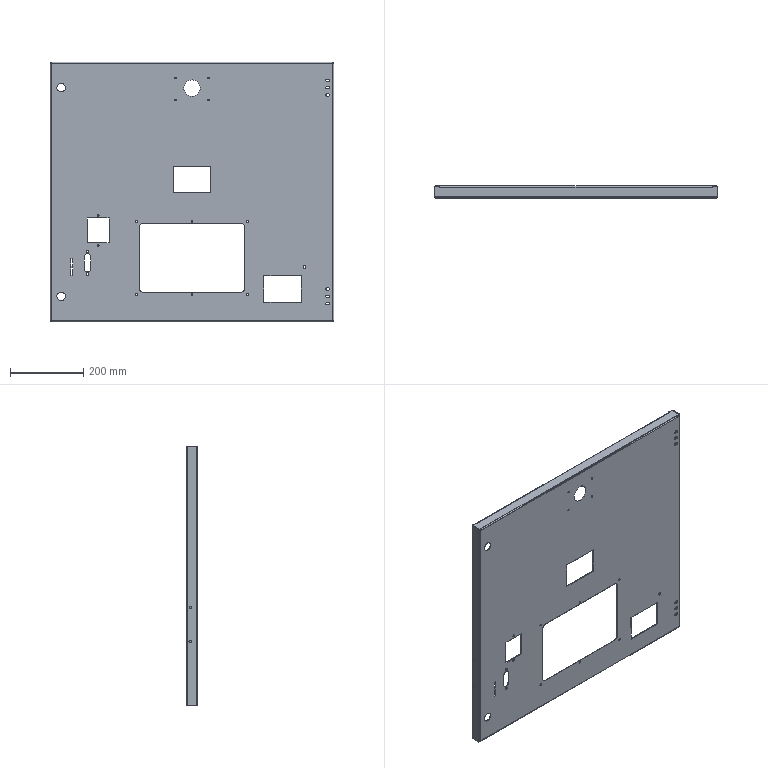Part | STEP file | 1 solid | 213 faces | box 775 x 32 x 710 mm | volume 1181727 mm3 | plane 133 | cylinder 80 | commonest cylinder face diameters 7 x30 5.3 x16 3 x10 4.2 x8 20.5 x4 23.5 x4